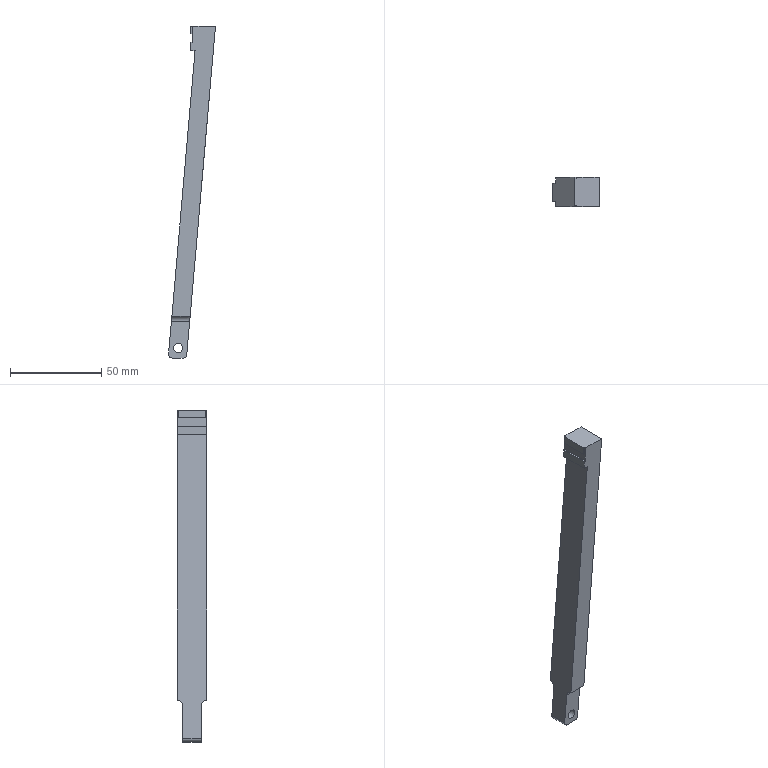Part | STEP file | solid 23 | 1 solid | 39 faces | box 25.771 x 16 x 182.341 mm | volume 28258 mm3 | plane 28 | cylinder 6 | other 4 | spline 1 | commonest cylinder face diameters 4 x2 6 x2 5 x1 6922 x1